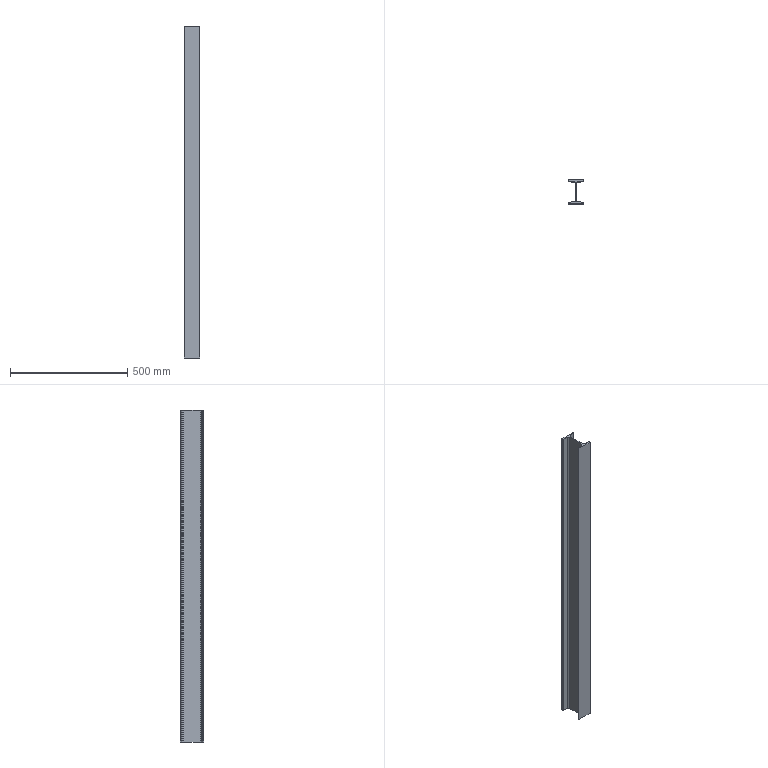Part | SolidWorks | features BaseBody 1 | 1 solid | 22 faces | box 67.6 x 101.6 x 1413 mm | volume 1963956 mm3 | plane 14 | cylinder 8 | commonest cylinder face diameters 5.6 x4 14.8 x4
STEP:
#1=CARTESIAN_POINT('',(45.812,22.014,0.));
#2=VERTEX_POINT('',#1);
#3=CARTESIAN_POINT('',(45.812,91.894,0.));
#4=VERTEX_POINT('',#3);
#5=CARTESIAN_POINT('',(45.812,91.894,0.));
#6=DIRECTION('',(0.,1.,0.));
#7=VECTOR('',#6,1000.);
#8=LINE('',#5,#7);
#9=EDGE_CURVE('',#2,#4,#8,.T.);
#10=ORIENTED_EDGE('',*,*,#9,.T.);
#11=CARTESIAN_POINT('',(45.812,91.894,1413.));
#12=VERTEX_POINT('',#11);
#13=CARTESIAN_POINT('',(45.812,91.894,0.));
#14=DIRECTION('',(0.,0.,1.));
#15=VECTOR('',#14,1000.);
#16=LINE('',#13,#15);
#17=EDGE_CURVE('',#4,#12,#16,.T.);
#18=ORIENTED_EDGE('',*,*,#17,.T.);
#19=CARTESIAN_POINT('',(45.812,22.014,1413.));
#20=VERTEX_POINT('',#19);
#21=CARTESIAN_POINT('',(45.812,91.894,1413.));
#22=DIRECTION('',(0.,-1.,0.));
#23=VECTOR('',#22,1000.);
#24=LINE('',#21,#23);
#25=EDGE_CURVE('',#12,#20,#24,.T.);
#26=ORIENTED_EDGE('',*,*,#25,.T.);
#27=CARTESIAN_POINT('',(45.812,22.014,0.));
#28=DIRECTION('',(0.,0.,-1.));
#29=VECTOR('',#28,1000.);
#30=LINE('',#27,#29);
#31=EDGE_CURVE('',#20,#2,#30,.T.);
#32=ORIENTED_EDGE('',*,*,#31,.T.);
#33=EDGE_LOOP('',(#10,#18,#26,#32));
#34=FACE_OUTER_BOUND('',#33,.T.);
#35=CARTESIAN_POINT('',(45.812,91.894,0.));
#36=DIRECTION('',(1.,0.,0.));
#37=DIRECTION('',(0.,0.,-1.));
#38=AXIS2_PLACEMENT_3D('',#35,#36,#37);
#39=PLANE('',#38);
#40=ADVANCED_FACE('',(#34),#39,.T.);
#41=ORIENTED_EDGE('',*,*,#17,.F.);
#42=CARTESIAN_POINT('',(51.991,99.193,0.));
#43=VERTEX_POINT('',#42);
#44=CARTESIAN_POINT('',(53.212,91.894,0.));
#45=DIRECTION('',(0.,0.,1.));
#46=DIRECTION('',(1.,0.,0.));
#47=AXIS2_PLACEMENT_3D('',#44,#45,#46);
#48=CIRCLE('',#47,7.4);
#49=EDGE_CURVE('',#43,#4,#48,.T.);
#50=ORIENTED_EDGE('',*,*,#49,.F.);
#51=CARTESIAN_POINT('',(51.991,99.193,1413.));
#52=VERTEX_POINT('',#51);
#53=CARTESIAN_POINT('',(51.991,99.193,0.));
#54=DIRECTION('',(0.,0.,-1.));
#55=VECTOR('',#54,1000.);
#56=LINE('',#53,#55);
#57=EDGE_CURVE('',#52,#43,#56,.T.);
#58=ORIENTED_EDGE('',*,*,#57,.F.);
#59=CARTESIAN_POINT('',(53.212,91.894,1413.));
#60=DIRECTION('',(0.,0.,-1.));
#61=DIRECTION('',(1.,0.,0.));
#62=AXIS2_PLACEMENT_3D('',#59,#60,#61);
#63=CIRCLE('',#62,7.4);
#64=EDGE_CURVE('',#12,#52,#63,.T.);
#65=ORIENTED_EDGE('',*,*,#64,.F.);
#66=EDGE_LOOP('',(#41,#50,#58,#65));
#67=FACE_OUTER_BOUND('',#66,.T.);
#68=CARTESIAN_POINT('',(53.212,91.894,0.));
#69=DIRECTION('',(0.,0.,1.));
#70=DIRECTION('',(1.,0.,0.));
#71=AXIS2_PLACEMENT_3D('',#68,#69,#70);
#72=CYLINDRICAL_SURFACE('',#71,7.4);
#73=ADVANCED_FACE('',(#67),#72,.F.);
#74=CARTESIAN_POINT('',(77.212,107.754,0.));
#75=VERTEX_POINT('',#74);
#76=CARTESIAN_POINT('',(9.612,107.754,0.));
#77=VERTEX_POINT('',#76);
#78=CARTESIAN_POINT('',(43.412,107.754,0.));
#79=DIRECTION('',(-1.,0.,0.));
#80=VECTOR('',#79,1000.);
#81=LINE('',#78,#80);
#82=EDGE_CURVE('',#75,#77,#81,.T.);
#83=ORIENTED_EDGE('',*,*,#82,.F.);
#84=CARTESIAN_POINT('',(77.212,105.784,0.));
#85=VERTEX_POINT('',#84);
#86=CARTESIAN_POINT('',(77.212,56.954,0.));
#87=DIRECTION('',(0.,1.,0.));
#88=VECTOR('',#87,1000.);
#89=LINE('',#86,#88);
#90=EDGE_CURVE('',#85,#75,#89,.T.);
#91=ORIENTED_EDGE('',*,*,#90,.F.);
#92=CARTESIAN_POINT('',(74.874,103.022,0.));
#93=VERTEX_POINT('',#92);
#94=CARTESIAN_POINT('',(74.412,105.784,0.));
#95=DIRECTION('',(0.,0.,1.));
#96=DIRECTION('',(1.,0.,0.));
#97=AXIS2_PLACEMENT_3D('',#94,#95,#96);
#98=CIRCLE('',#97,2.8);
#99=EDGE_CURVE('',#93,#85,#98,.T.);
#100=ORIENTED_EDGE('',*,*,#99,.F.);
#101=CARTESIAN_POINT('',(51.991,99.193,0.));
#102=DIRECTION('',(0.9863,0.165,0.));
#103=VECTOR('',#102,1000.);
#104=LINE('',#101,#103);
#105=EDGE_CURVE('',#43,#93,#104,.T.);
#106=ORIENTED_EDGE('',*,*,#105,.F.);
#107=ORIENTED_EDGE('',*,*,#49,.T.);
#108=ORIENTED_EDGE('',*,*,#9,.F.);
#109=CARTESIAN_POINT('',(51.991,14.716,0.));
#110=VERTEX_POINT('',#109);
#111=CARTESIAN_POINT('',(53.212,22.014,0.));
#112=DIRECTION('',(0.,0.,-1.));
#113=DIRECTION('',(1.,0.,0.));
#114=AXIS2_PLACEMENT_3D('',#111,#112,#113);
#115=CIRCLE('',#114,7.4);
#116=EDGE_CURVE('',#110,#2,#115,.T.);
#117=ORIENTED_EDGE('',*,*,#116,.F.);
#118=CARTESIAN_POINT('',(74.874,10.886,0.));
#119=VERTEX_POINT('',#118);
#120=CARTESIAN_POINT('',(74.874,10.886,0.));
#121=DIRECTION('',(-0.9863,0.165,0.));
#122=VECTOR('',#121,1000.);
#123=LINE('',#120,#122);
#124=EDGE_CURVE('',#119,#110,#123,.T.);
#125=ORIENTED_EDGE('',*,*,#124,.F.);
#126=CARTESIAN_POINT('',(77.212,8.125,0.));
#127=VERTEX_POINT('',#126);
#128=CARTESIAN_POINT('',(74.412,8.125,0.));
#129=DIRECTION('',(0.,0.,1.));
#130=DIRECTION('',(1.,0.,0.));
#131=AXIS2_PLACEMENT_3D('',#128,#129,#130);
#132=CIRCLE('',#131,2.8);
#133=EDGE_CURVE('',#127,#119,#132,.T.);
#134=ORIENTED_EDGE('',*,*,#133,.F.);
#135=CARTESIAN_POINT('',(77.212,6.154,0.));
#136=VERTEX_POINT('',#135);
#137=CARTESIAN_POINT('',(77.212,56.954,0.));
#138=DIRECTION('',(0.,1.,0.));
#139=VECTOR('',#138,1000.);
#140=LINE('',#137,#139);
#141=EDGE_CURVE('',#136,#127,#140,.T.);
#142=ORIENTED_EDGE('',*,*,#141,.F.);
#143=CARTESIAN_POINT('',(9.612,6.154,0.));
#144=VERTEX_POINT('',#143);
#145=CARTESIAN_POINT('',(43.412,6.154,0.));
#146=DIRECTION('',(1.,0.,0.));
#147=VECTOR('',#146,1000.);
#148=LINE('',#145,#147);
#149=EDGE_CURVE('',#144,#136,#148,.T.);
#150=ORIENTED_EDGE('',*,*,#149,.F.);
#151=CARTESIAN_POINT('',(9.612,8.125,0.));
#152=VERTEX_POINT('',#151);
#153=CARTESIAN_POINT('',(9.612,56.954,0.));
#154=DIRECTION('',(0.,-1.,0.));
#155=VECTOR('',#154,1000.);
#156=LINE('',#153,#155);
#157=EDGE_CURVE('',#152,#144,#156,.T.);
#158=ORIENTED_EDGE('',*,*,#157,.F.);
#159=CARTESIAN_POINT('',(11.95,10.886,0.));
#160=VERTEX_POINT('',#159);
#161=CARTESIAN_POINT('',(12.412,8.125,0.));
#162=DIRECTION('',(0.,0.,1.));
#163=DIRECTION('',(1.,0.,0.));
#164=AXIS2_PLACEMENT_3D('',#161,#162,#163);
#165=CIRCLE('',#164,2.8);
#166=EDGE_CURVE('',#160,#152,#165,.T.);
#167=ORIENTED_EDGE('',*,*,#166,.F.);
#168=CARTESIAN_POINT('',(34.833,14.716,0.));
#169=VERTEX_POINT('',#168);
#170=CARTESIAN_POINT('',(34.833,14.716,0.));
#171=DIRECTION('',(-0.9863,-0.165,0.));
#172=VECTOR('',#171,1000.);
#173=LINE('',#170,#172);
#174=EDGE_CURVE('',#169,#160,#173,.T.);
#175=ORIENTED_EDGE('',*,*,#174,.F.);
#176=CARTESIAN_POINT('',(41.012,22.014,0.));
#177=VERTEX_POINT('',#176);
#178=CARTESIAN_POINT('',(33.612,22.014,0.));
#179=DIRECTION('',(0.,0.,-1.));
#180=DIRECTION('',(1.,0.,0.));
#181=AXIS2_PLACEMENT_3D('',#178,#179,#180);
#182=CIRCLE('',#181,7.4);
#183=EDGE_CURVE('',#177,#169,#182,.T.);
#184=ORIENTED_EDGE('',*,*,#183,.F.);
#185=CARTESIAN_POINT('',(41.012,91.894,0.));
#186=VERTEX_POINT('',#185);
#187=CARTESIAN_POINT('',(41.012,56.954,0.));
#188=DIRECTION('',(0.,-1.,0.));
#189=VECTOR('',#188,1000.);
#190=LINE('',#187,#189);
#191=EDGE_CURVE('',#186,#177,#190,.T.);
#192=ORIENTED_EDGE('',*,*,#191,.F.);
#193=CARTESIAN_POINT('',(34.833,99.193,0.));
#194=VERTEX_POINT('',#193);
#195=CARTESIAN_POINT('',(33.612,91.894,0.));
#196=DIRECTION('',(0.,0.,-1.));
#197=DIRECTION('',(1.,0.,0.));
#198=AXIS2_PLACEMENT_3D('',#195,#196,#197);
#199=CIRCLE('',#198,7.4);
#200=EDGE_CURVE('',#194,#186,#199,.T.);
#201=ORIENTED_EDGE('',*,*,#200,.F.);
#202=CARTESIAN_POINT('',(11.95,103.022,0.));
#203=VERTEX_POINT('',#202);
#204=CARTESIAN_POINT('',(11.95,103.022,0.));
#205=DIRECTION('',(0.9863,-0.165,0.));
#206=VECTOR('',#205,1000.);
#207=LINE('',#204,#206);
#208=EDGE_CURVE('',#203,#194,#207,.T.);
#209=ORIENTED_EDGE('',*,*,#208,.F.);
#210=CARTESIAN_POINT('',(9.612,105.784,0.));
#211=VERTEX_POINT('',#210);
#212=CARTESIAN_POINT('',(12.412,105.784,0.));
#213=DIRECTION('',(0.,0.,1.));
#214=DIRECTION('',(1.,0.,0.));
#215=AXIS2_PLACEMENT_3D('',#212,#213,#214);
#216=CIRCLE('',#215,2.8);
#217=EDGE_CURVE('',#211,#203,#216,.T.);
#218=ORIENTED_EDGE('',*,*,#217,.F.);
#219=CARTESIAN_POINT('',(9.612,56.954,0.));
#220=DIRECTION('',(0.,-1.,0.));
#221=VECTOR('',#220,1000.);
#222=LINE('',#219,#221);
#223=EDGE_CURVE('',#77,#211,#222,.T.);
#224=ORIENTED_EDGE('',*,*,#223,.F.);
#225=EDGE_LOOP('',(#83,#91,#100,#106,#107,#108,#117,#125,#134,#142,#150,#158,#167,#175,#184,#192,#201,#209,#218,#224));
#226=FACE_OUTER_BOUND('',#225,.T.);
#227=CARTESIAN_POINT('',(43.412,56.954,0.));
#228=DIRECTION('',(0.,0.,1.));
#229=DIRECTION('',(1.,0.,0.));
#230=AXIS2_PLACEMENT_3D('',#227,#228,#229);
#231=PLANE('',#230);
#232=ADVANCED_FACE('',(#226),#231,.F.);
#233=CARTESIAN_POINT('',(51.991,14.716,1413.));
#234=VERTEX_POINT('',#233);
#235=CARTESIAN_POINT('',(51.991,14.716,0.));
#236=DIRECTION('',(0.,0.,1.));
#237=VECTOR('',#236,1000.);
#238=LINE('',#235,#237);
#239=EDGE_CURVE('',#110,#234,#238,.T.);
#240=ORIENTED_EDGE('',*,*,#239,.F.);
#241=ORIENTED_EDGE('',*,*,#116,.T.);
#242=ORIENTED_EDGE('',*,*,#31,.F.);
#243=CARTESIAN_POINT('',(53.212,22.014,1413.));
#244=DIRECTION('',(0.,0.,-1.));
#245=DIRECTION('',(1.,0.,0.));
#246=AXIS2_PLACEMENT_3D('',#243,#244,#245);
#247=CIRCLE('',#246,7.4);
#248=EDGE_CURVE('',#234,#20,#247,.T.);
#249=ORIENTED_EDGE('',*,*,#248,.F.);
#250=EDGE_LOOP('',(#240,#241,#242,#249));
#251=FACE_OUTER_BOUND('',#250,.T.);
#252=CARTESIAN_POINT('',(53.212,22.014,0.));
#253=DIRECTION('',(0.,0.,1.));
#254=DIRECTION('',(1.,0.,0.));
#255=AXIS2_PLACEMENT_3D('',#252,#253,#254);
#256=CYLINDRICAL_SURFACE('',#255,7.4);
#257=ADVANCED_FACE('',(#251),#256,.F.);
#258=CARTESIAN_POINT('',(74.874,103.022,1413.));
#259=VERTEX_POINT('',#258);
#260=CARTESIAN_POINT('',(77.212,105.784,1413.));
#261=VERTEX_POINT('',#260);
#262=CARTESIAN_POINT('',(74.412,105.784,1413.));
#263=DIRECTION('',(0.,0.,1.));
#264=DIRECTION('',(1.,0.,0.));
#265=AXIS2_PLACEMENT_3D('',#262,#263,#264);
#266=CIRCLE('',#265,2.8);
#267=EDGE_CURVE('',#259,#261,#266,.T.);
#268=ORIENTED_EDGE('',*,*,#267,.T.);
#269=CARTESIAN_POINT('',(77.212,107.754,1413.));
#270=VERTEX_POINT('',#269);
#271=CARTESIAN_POINT('',(77.212,56.954,1413.));
#272=DIRECTION('',(0.,1.,0.));
#273=VECTOR('',#272,1000.);
#274=LINE('',#271,#273);
#275=EDGE_CURVE('',#261,#270,#274,.T.);
#276=ORIENTED_EDGE('',*,*,#275,.T.);
#277=CARTESIAN_POINT('',(9.612,107.754,1413.));
#278=VERTEX_POINT('',#277);
#279=CARTESIAN_POINT('',(43.412,107.754,1413.));
#280=DIRECTION('',(-1.,0.,0.));
#281=VECTOR('',#280,1000.);
#282=LINE('',#279,#281);
#283=EDGE_CURVE('',#270,#278,#282,.T.);
#284=ORIENTED_EDGE('',*,*,#283,.T.);
#285=CARTESIAN_POINT('',(9.612,105.784,1413.));
#286=VERTEX_POINT('',#285);
#287=CARTESIAN_POINT('',(9.612,56.954,1413.));
#288=DIRECTION('',(0.,-1.,0.));
#289=VECTOR('',#288,1000.);
#290=LINE('',#287,#289);
#291=EDGE_CURVE('',#278,#286,#290,.T.);
#292=ORIENTED_EDGE('',*,*,#291,.T.);
#293=CARTESIAN_POINT('',(11.95,103.022,1413.));
#294=VERTEX_POINT('',#293);
#295=CARTESIAN_POINT('',(12.412,105.784,1413.));
#296=DIRECTION('',(0.,0.,1.));
#297=DIRECTION('',(1.,0.,0.));
#298=AXIS2_PLACEMENT_3D('',#295,#296,#297);
#299=CIRCLE('',#298,2.8);
#300=EDGE_CURVE('',#286,#294,#299,.T.);
#301=ORIENTED_EDGE('',*,*,#300,.T.);
#302=CARTESIAN_POINT('',(34.833,99.193,1413.));
#303=VERTEX_POINT('',#302);
#304=CARTESIAN_POINT('',(11.95,103.022,1413.));
#305=DIRECTION('',(0.9863,-0.165,0.));
#306=VECTOR('',#305,1000.);
#307=LINE('',#304,#306);
#308=EDGE_CURVE('',#294,#303,#307,.T.);
#309=ORIENTED_EDGE('',*,*,#308,.T.);
#310=CARTESIAN_POINT('',(41.012,91.894,1413.));
#311=VERTEX_POINT('',#310);
#312=CARTESIAN_POINT('',(33.612,91.894,1413.));
#313=DIRECTION('',(0.,0.,-1.));
#314=DIRECTION('',(1.,0.,0.));
#315=AXIS2_PLACEMENT_3D('',#312,#313,#314);
#316=CIRCLE('',#315,7.4);
#317=EDGE_CURVE('',#303,#311,#316,.T.);
#318=ORIENTED_EDGE('',*,*,#317,.T.);
#319=CARTESIAN_POINT('',(41.012,22.014,1413.));
#320=VERTEX_POINT('',#319);
#321=CARTESIAN_POINT('',(41.012,56.954,1413.));
#322=DIRECTION('',(0.,-1.,0.));
#323=VECTOR('',#322,1000.);
#324=LINE('',#321,#323);
#325=EDGE_CURVE('',#311,#320,#324,.T.);
#326=ORIENTED_EDGE('',*,*,#325,.T.);
#327=CARTESIAN_POINT('',(34.833,14.716,1413.));
#328=VERTEX_POINT('',#327);
#329=CARTESIAN_POINT('',(33.612,22.014,1413.));
#330=DIRECTION('',(0.,0.,-1.));
#331=DIRECTION('',(1.,0.,0.));
#332=AXIS2_PLACEMENT_3D('',#329,#330,#331);
#333=CIRCLE('',#332,7.4);
#334=EDGE_CURVE('',#320,#328,#333,.T.);
#335=ORIENTED_EDGE('',*,*,#334,.T.);
#336=CARTESIAN_POINT('',(11.95,10.886,1413.));
#337=VERTEX_POINT('',#336);
#338=CARTESIAN_POINT('',(34.833,14.716,1413.));
#339=DIRECTION('',(-0.9863,-0.165,0.));
#340=VECTOR('',#339,1000.);
#341=LINE('',#338,#340);
#342=EDGE_CURVE('',#328,#337,#341,.T.);
#343=ORIENTED_EDGE('',*,*,#342,.T.);
#344=CARTESIAN_POINT('',(9.612,8.125,1413.));
#345=VERTEX_POINT('',#344);
#346=CARTESIAN_POINT('',(12.412,8.125,1413.));
#347=DIRECTION('',(0.,0.,1.));
#348=DIRECTION('',(1.,0.,0.));
#349=AXIS2_PLACEMENT_3D('',#346,#347,#348);
#350=CIRCLE('',#349,2.8);
#351=EDGE_CURVE('',#337,#345,#350,.T.);
#352=ORIENTED_EDGE('',*,*,#351,.T.);
#353=CARTESIAN_POINT('',(9.612,6.154,1413.));
#354=VERTEX_POINT('',#353);
#355=CARTESIAN_POINT('',(9.612,56.954,1413.));
#356=DIRECTION('',(0.,-1.,0.));
#357=VECTOR('',#356,1000.);
#358=LINE('',#355,#357);
#359=EDGE_CURVE('',#345,#354,#358,.T.);
#360=ORIENTED_EDGE('',*,*,#359,.T.);
#361=CARTESIAN_POINT('',(77.212,6.154,1413.));
#362=VERTEX_POINT('',#361);
#363=CARTESIAN_POINT('',(43.412,6.154,1413.));
#364=DIRECTION('',(1.,0.,0.));
#365=VECTOR('',#364,1000.);
#366=LINE('',#363,#365);
#367=EDGE_CURVE('',#354,#362,#366,.T.);
#368=ORIENTED_EDGE('',*,*,#367,.T.);
#369=CARTESIAN_POINT('',(77.212,8.125,1413.));
#370=VERTEX_POINT('',#369);
#371=CARTESIAN_POINT('',(77.212,56.954,1413.));
#372=DIRECTION('',(0.,1.,0.));
#373=VECTOR('',#372,1000.);
#374=LINE('',#371,#373);
#375=EDGE_CURVE('',#362,#370,#374,.T.);
#376=ORIENTED_EDGE('',*,*,#375,.T.);
#377=CARTESIAN_POINT('',(74.874,10.886,1413.));
#378=VERTEX_POINT('',#377);
#379=CARTESIAN_POINT('',(74.412,8.125,1413.));
#380=DIRECTION('',(0.,0.,1.));
#381=DIRECTION('',(1.,0.,0.));
#382=AXIS2_PLACEMENT_3D('',#379,#380,#381);
#383=CIRCLE('',#382,2.8);
#384=EDGE_CURVE('',#370,#378,#383,.T.);
#385=ORIENTED_EDGE('',*,*,#384,.T.);
#386=CARTESIAN_POINT('',(74.874,10.886,1413.));
#387=DIRECTION('',(-0.9863,0.165,0.));
#388=VECTOR('',#387,1000.);
#389=LINE('',#386,#388);
#390=EDGE_CURVE('',#378,#234,#389,.T.);
#391=ORIENTED_EDGE('',*,*,#390,.T.);
#392=ORIENTED_EDGE('',*,*,#248,.T.);
#393=ORIENTED_EDGE('',*,*,#25,.F.);
#394=ORIENTED_EDGE('',*,*,#64,.T.);
#395=CARTESIAN_POINT('',(51.991,99.193,1413.));
#396=DIRECTION('',(0.9863,0.165,0.));
#397=VECTOR('',#396,1000.);
#398=LINE('',#395,#397);
#399=EDGE_CURVE('',#52,#259,#398,.T.);
#400=ORIENTED_EDGE('',*,*,#399,.T.);
#401=EDGE_LOOP('',(#268,#276,#284,#292,#301,#309,#318,#326,#335,#343,#352,#360,#368,#376,#385,#391,#392,#393,#394,#400));
#402=FACE_OUTER_BOUND('',#401,.T.);
#403=CARTESIAN_POINT('',(43.412,56.954,1413.));
#404=DIRECTION('',(0.,0.,1.));
#405=DIRECTION('',(1.,0.,0.));
#406=AXIS2_PLACEMENT_3D('',#403,#404,#405);
#407=PLANE('',#406);
#408=ADVANCED_FACE('',(#402),#407,.T.);
#409=ORIENTED_EDGE('',*,*,#105,.T.);
#410=CARTESIAN_POINT('',(74.874,103.022,0.));
#411=DIRECTION('',(0.,0.,1.));
#412=VECTOR('',#411,1000.);
#413=LINE('',#410,#412);
#414=EDGE_CURVE('',#93,#259,#413,.T.);
#415=ORIENTED_EDGE('',*,*,#414,.T.);
#416=ORIENTED_EDGE('',*,*,#399,.F.);
#417=ORIENTED_EDGE('',*,*,#57,.T.);
#418=EDGE_LOOP('',(#409,#415,#416,#417));
#419=FACE_OUTER_BOUND('',#418,.T.);
#420=CARTESIAN_POINT('',(74.874,103.022,0.));
#421=DIRECTION('',(0.165,-0.9863,0.));
#422=DIRECTION('',(0.9863,0.165,0.));
#423=AXIS2_PLACEMENT_3D('',#420,#421,#422);
#424=PLANE('',#423);
#425=ADVANCED_FACE('',(#419),#424,.T.);
#426=ORIENTED_EDGE('',*,*,#223,.T.);
#427=CARTESIAN_POINT('',(9.612,105.784,0.));
#428=DIRECTION('',(0.,0.,1.));
#429=VECTOR('',#428,1000.);
#430=LINE('',#427,#429);
#431=EDGE_CURVE('',#211,#286,#430,.T.);
#432=ORIENTED_EDGE('',*,*,#431,.T.);
#433=ORIENTED_EDGE('',*,*,#291,.F.);
#434=CARTESIAN_POINT('',(9.612,107.754,0.));
#435=DIRECTION('',(0.,0.,-1.));
#436=VECTOR('',#435,1000.);
#437=LINE('',#434,#436);
#438=EDGE_CURVE('',#278,#77,#437,.T.);
#439=ORIENTED_EDGE('',*,*,#438,.T.);
#440=EDGE_LOOP('',(#426,#432,#433,#439));
#441=FACE_OUTER_BOUND('',#440,.T.);
#442=CARTESIAN_POINT('',(9.612,105.784,0.));
#443=DIRECTION('',(-1.,0.,0.));
#444=DIRECTION('',(0.,0.,1.));
#445=AXIS2_PLACEMENT_3D('',#442,#443,#444);
#446=PLANE('',#445);
#447=ADVANCED_FACE('',(#441),#446,.T.);
#448=ORIENTED_EDGE('',*,*,#82,.T.);
#449=ORIENTED_EDGE('',*,*,#438,.F.);
#450=ORIENTED_EDGE('',*,*,#283,.F.);
#451=CARTESIAN_POINT('',(77.212,107.754,0.));
#452=DIRECTION('',(0.,0.,-1.));
#453=VECTOR('',#452,1000.);
#454=LINE('',#451,#453);
#455=EDGE_CURVE('',#270,#75,#454,.T.);
#456=ORIENTED_EDGE('',*,*,#455,.T.);
#457=EDGE_LOOP('',(#448,#449,#450,#456));
#458=FACE_OUTER_BOUND('',#457,.T.);
#459=CARTESIAN_POINT('',(9.612,107.754,0.));
#460=DIRECTION('',(0.,1.,0.));
#461=DIRECTION('',(0.,0.,1.));
#462=AXIS2_PLACEMENT_3D('',#459,#460,#461);
#463=PLANE('',#462);
#464=ADVANCED_FACE('',(#458),#463,.T.);
#465=ORIENTED_EDGE('',*,*,#90,.T.);
#466=ORIENTED_EDGE('',*,*,#455,.F.);
#467=ORIENTED_EDGE('',*,*,#275,.F.);
#468=CARTESIAN_POINT('',(77.212,105.784,0.));
#469=DIRECTION('',(0.,0.,-1.));
#470=VECTOR('',#469,1000.);
#471=LINE('',#468,#470);
#472=EDGE_CURVE('',#261,#85,#471,.T.);
#473=ORIENTED_EDGE('',*,*,#472,.T.);
#474=EDGE_LOOP('',(#465,#466,#467,#473));
#475=FACE_OUTER_BOUND('',#474,.T.);
#476=CARTESIAN_POINT('',(77.212,107.754,0.));
#477=DIRECTION('',(1.,0.,0.));
#478=DIRECTION('',(0.,1.,0.));
#479=AXIS2_PLACEMENT_3D('',#476,#477,#478);
#480=PLANE('',#479);
#481=ADVANCED_FACE('',(#475),#480,.T.);
#482=ORIENTED_EDGE('',*,*,#99,.T.);
#483=ORIENTED_EDGE('',*,*,#472,.F.);
#484=ORIENTED_EDGE('',*,*,#267,.F.);
#485=ORIENTED_EDGE('',*,*,#414,.F.);
#486=EDGE_LOOP('',(#482,#483,#484,#485));
#487=FACE_OUTER_BOUND('',#486,.T.);
#488=CARTESIAN_POINT('',(74.412,105.784,0.));
#489=DIRECTION('',(0.,0.,1.));
#490=DIRECTION('',(1.,0.,0.));
#491=AXIS2_PLACEMENT_3D('',#488,#489,#490);
#492=CYLINDRICAL_SURFACE('',#491,2.8);
#493=ADVANCED_FACE('',(#487),#492,.T.);
#494=ORIENTED_EDGE('',*,*,#124,.T.);
#495=ORIENTED_EDGE('',*,*,#239,.T.);
#496=ORIENTED_EDGE('',*,*,#390,.F.);
#497=CARTESIAN_POINT('',(74.874,10.886,0.));
#498=DIRECTION('',(0.,0.,-1.));
#499=VECTOR('',#498,1000.);
#500=LINE('',#497,#499);
#501=EDGE_CURVE('',#378,#119,#500,.T.);
#502=ORIENTED_EDGE('',*,*,#501,.T.);
#503=EDGE_LOOP('',(#494,#495,#496,#502));
#504=FACE_OUTER_BOUND('',#503,.T.);
#505=CARTESIAN_POINT('',(51.991,14.716,0.));
#506=DIRECTION('',(0.165,0.9863,0.));
#507=DIRECTION('',(-0.9863,0.165,0.));
#508=AXIS2_PLACEMENT_3D('',#505,#506,#507);
#509=PLANE('',#508);
#510=ADVANCED_FACE('',(#504),#509,.T.);
#511=ORIENTED_EDGE('',*,*,#133,.T.);
#512=ORIENTED_EDGE('',*,*,#501,.F.);
#513=ORIENTED_EDGE('',*,*,#384,.F.);
#514=CARTESIAN_POINT('',(77.212,8.125,0.));
#515=DIRECTION('',(0.,0.,-1.));
#516=VECTOR('',#515,1000.);
#517=LINE('',#514,#516);
#518=EDGE_CURVE('',#370,#127,#517,.T.);
#519=ORIENTED_EDGE('',*,*,#518,.T.);
#520=EDGE_LOOP('',(#511,#512,#513,#519));
#521=FACE_OUTER_BOUND('',#520,.T.);
#522=CARTESIAN_POINT('',(74.412,8.125,0.));
#523=DIRECTION('',(0.,0.,1.));
#524=DIRECTION('',(1.,0.,0.));
#525=AXIS2_PLACEMENT_3D('',#522,#523,#524);
#526=CYLINDRICAL_SURFACE('',#525,2.8);
#527=ADVANCED_FACE('',(#521),#526,.T.);
#528=ORIENTED_EDGE('',*,*,#141,.T.);
#529=ORIENTED_EDGE('',*,*,#518,.F.);
#530=ORIENTED_EDGE('',*,*,#375,.F.);
#531=CARTESIAN_POINT('',(77.212,6.154,0.));
#532=DIRECTION('',(0.,0.,-1.));
#533=VECTOR('',#532,1000.);
#534=LINE('',#531,#533);
#535=EDGE_CURVE('',#362,#136,#534,.T.);
#536=ORIENTED_EDGE('',*,*,#535,.T.);
#537=EDGE_LOOP('',(#528,#529,#530,#536));
#538=FACE_OUTER_BOUND('',#537,.T.);
#539=CARTESIAN_POINT('',(77.212,8.125,0.));
#540=DIRECTION('',(1.,0.,0.));
#541=DIRECTION('',(0.,1.,0.));
#542=AXIS2_PLACEMENT_3D('',#539,#540,#541);
#543=PLANE('',#542);
#544=ADVANCED_FACE('',(#538),#543,.T.);
#545=ORIENTED_EDGE('',*,*,#149,.T.);
#546=ORIENTED_EDGE('',*,*,#535,.F.);
#547=ORIENTED_EDGE('',*,*,#367,.F.);
#548=CARTESIAN_POINT('',(9.612,6.154,0.));
#549=DIRECTION('',(0.,0.,-1.));
#550=VECTOR('',#549,1000.);
#551=LINE('',#548,#550);
#552=EDGE_CURVE('',#354,#144,#551,.T.);
#553=ORIENTED_EDGE('',*,*,#552,.T.);
#554=EDGE_LOOP('',(#545,#546,#547,#553));
#555=FACE_OUTER_BOUND('',#554,.T.);
#556=CARTESIAN_POINT('',(77.212,6.154,0.));
#557=DIRECTION('',(0.,-1.,0.));
#558=DIRECTION('',(0.,0.,-1.));
#559=AXIS2_PLACEMENT_3D('',#556,#557,#558);
#560=PLANE('',#559);
#561=ADVANCED_FACE('',(#555),#560,.T.);
#562=ORIENTED_EDGE('',*,*,#157,.T.);
#563=ORIENTED_EDGE('',*,*,#552,.F.);
#564=ORIENTED_EDGE('',*,*,#359,.F.);
#565=CARTESIAN_POINT('',(9.612,8.125,0.));
#566=DIRECTION('',(0.,0.,-1.));
#567=VECTOR('',#566,1000.);
#568=LINE('',#565,#567);
#569=EDGE_CURVE('',#345,#152,#568,.T.);
#570=ORIENTED_EDGE('',*,*,#569,.T.);
#571=EDGE_LOOP('',(#562,#563,#564,#570));
#572=FACE_OUTER_BOUND('',#571,.T.);
#573=CARTESIAN_POINT('',(9.612,6.154,0.));
#574=DIRECTION('',(-1.,0.,0.));
#575=DIRECTION('',(0.,-1.,0.));
#576=AXIS2_PLACEMENT_3D('',#573,#574,#575);
#577=PLANE('',#576);
#578=ADVANCED_FACE('',(#572),#577,.T.);
#579=ORIENTED_EDGE('',*,*,#166,.T.);
#580=ORIENTED_EDGE('',*,*,#569,.F.);
#581=ORIENTED_EDGE('',*,*,#351,.F.);
#582=CARTESIAN_POINT('',(11.95,10.886,0.));
#583=DIRECTION('',(0.,0.,-1.));
#584=VECTOR('',#583,1000.);
#585=LINE('',#582,#584);
#586=EDGE_CURVE('',#337,#160,#585,.T.);
#587=ORIENTED_EDGE('',*,*,#586,.T.);
#588=EDGE_LOOP('',(#579,#580,#581,#587));
#589=FACE_OUTER_BOUND('',#588,.T.);
#590=CARTESIAN_POINT('',(12.412,8.125,0.));
#591=DIRECTION('',(0.,0.,1.));
#592=DIRECTION('',(1.,0.,0.));
#593=AXIS2_PLACEMENT_3D('',#590,#591,#592);
#594=CYLINDRICAL_SURFACE('',#593,2.8);
#595=ADVANCED_FACE('',(#589),#594,.T.);
#596=ORIENTED_EDGE('',*,*,#174,.T.);
#597=ORIENTED_EDGE('',*,*,#586,.F.);
#598=ORIENTED_EDGE('',*,*,#342,.F.);
#599=CARTESIAN_POINT('',(34.833,14.716,0.));
#600=DIRECTION('',(0.,0.,-1.));
#601=VECTOR('',#600,1000.);
#602=LINE('',#599,#601);
#603=EDGE_CURVE('',#328,#169,#602,.T.);
#604=ORIENTED_EDGE('',*,*,#603,.T.);
#605=EDGE_LOOP('',(#596,#597,#598,#604));
#606=FACE_OUTER_BOUND('',#605,.T.);
#607=CARTESIAN_POINT('',(11.95,10.886,0.));
#608=DIRECTION('',(-0.165,0.9863,0.));
#609=DIRECTION('',(-0.9863,-0.165,0.));
#610=AXIS2_PLACEMENT_3D('',#607,#608,#609);
#611=PLANE('',#610);
#612=ADVANCED_FACE('',(#606),#611,.T.);
#613=CARTESIAN_POINT('',(41.012,22.014,0.));
#614=DIRECTION('',(0.,0.,1.));
#615=VECTOR('',#614,1000.);
#616=LINE('',#613,#615);
#617=EDGE_CURVE('',#177,#320,#616,.T.);
#618=ORIENTED_EDGE('',*,*,#617,.F.);
#619=ORIENTED_EDGE('',*,*,#183,.T.);
#620=ORIENTED_EDGE('',*,*,#603,.F.);
#621=ORIENTED_EDGE('',*,*,#334,.F.);
#622=EDGE_LOOP('',(#618,#619,#620,#621));
#623=FACE_OUTER_BOUND('',#622,.T.);
#624=CARTESIAN_POINT('',(33.612,22.014,0.));
#625=DIRECTION('',(0.,0.,1.));
#626=DIRECTION('',(1.,0.,0.));
#627=AXIS2_PLACEMENT_3D('',#624,#625,#626);
#628=CYLINDRICAL_SURFACE('',#627,7.4);
#629=ADVANCED_FACE('',(#623),#628,.F.);
#630=ORIENTED_EDGE('',*,*,#191,.T.);
#631=ORIENTED_EDGE('',*,*,#617,.T.);
#632=ORIENTED_EDGE('',*,*,#325,.F.);
#633=CARTESIAN_POINT('',(41.012,91.894,0.));
#634=DIRECTION('',(0.,0.,-1.));
#635=VECTOR('',#634,1000.);
#636=LINE('',#633,#635);
#637=EDGE_CURVE('',#311,#186,#636,.T.);
#638=ORIENTED_EDGE('',*,*,#637,.T.);
#639=EDGE_LOOP('',(#630,#631,#632,#638));
#640=FACE_OUTER_BOUND('',#639,.T.);
#641=CARTESIAN_POINT('',(41.012,22.014,0.));
#642=DIRECTION('',(-1.,0.,0.));
#643=DIRECTION('',(0.,0.,1.));
#644=AXIS2_PLACEMENT_3D('',#641,#642,#643);
#645=PLANE('',#644);
#646=ADVANCED_FACE('',(#640),#645,.T.);
#647=CARTESIAN_POINT('',(34.833,99.193,0.));
#648=DIRECTION('',(0.,0.,1.));
#649=VECTOR('',#648,1000.);
#650=LINE('',#647,#649);
#651=EDGE_CURVE('',#194,#303,#650,.T.);
#652=ORIENTED_EDGE('',*,*,#651,.F.);
#653=ORIENTED_EDGE('',*,*,#200,.T.);
#654=ORIENTED_EDGE('',*,*,#637,.F.);
#655=ORIENTED_EDGE('',*,*,#317,.F.);
#656=EDGE_LOOP('',(#652,#653,#654,#655));
#657=FACE_OUTER_BOUND('',#656,.T.);
#658=CARTESIAN_POINT('',(33.612,91.894,0.));
#659=DIRECTION('',(0.,0.,1.));
#660=DIRECTION('',(1.,0.,0.));
#661=AXIS2_PLACEMENT_3D('',#658,#659,#660);
#662=CYLINDRICAL_SURFACE('',#661,7.4);
#663=ADVANCED_FACE('',(#657),#662,.F.);
#664=ORIENTED_EDGE('',*,*,#208,.T.);
#665=ORIENTED_EDGE('',*,*,#651,.T.);
#666=ORIENTED_EDGE('',*,*,#308,.F.);
#667=CARTESIAN_POINT('',(11.95,103.022,0.));
#668=DIRECTION('',(0.,0.,-1.));
#669=VECTOR('',#668,1000.);
#670=LINE('',#667,#669);
#671=EDGE_CURVE('',#294,#203,#670,.T.);
#672=ORIENTED_EDGE('',*,*,#671,.T.);
#673=EDGE_LOOP('',(#664,#665,#666,#672));
#674=FACE_OUTER_BOUND('',#673,.T.);
#675=CARTESIAN_POINT('',(34.833,99.193,0.));
#676=DIRECTION('',(-0.165,-0.9863,0.));
#677=DIRECTION('',(0.9863,-0.165,0.));
#678=AXIS2_PLACEMENT_3D('',#675,#676,#677);
#679=PLANE('',#678);
#680=ADVANCED_FACE('',(#674),#679,.T.);
#681=ORIENTED_EDGE('',*,*,#217,.T.);
#682=ORIENTED_EDGE('',*,*,#671,.F.);
#683=ORIENTED_EDGE('',*,*,#300,.F.);
#684=ORIENTED_EDGE('',*,*,#431,.F.);
#685=EDGE_LOOP('',(#681,#682,#683,#684));
#686=FACE_OUTER_BOUND('',#685,.T.);
#687=CARTESIAN_POINT('',(12.412,105.784,0.));
#688=DIRECTION('',(0.,0.,1.));
#689=DIRECTION('',(1.,0.,0.));
#690=AXIS2_PLACEMENT_3D('',#687,#688,#689);
#691=CYLINDRICAL_SURFACE('',#690,2.8);
#692=ADVANCED_FACE('',(#686),#691,.T.);
#693=CLOSED_SHELL('',(#40,#73,#232,#257,#408,#425,#447,#464,#481,#493,#510,#527,#544,#561,#578,#595,#612,#629,#646,#663,#680,#692));
#694=MANIFOLD_SOLID_BREP('',#693);
#695=CARTESIAN_POINT('',(0.,0.,0.));
#696=DIRECTION('',(0.,0.,1.));
#697=DIRECTION('',(1.,0.,0.));
#698=AXIS2_PLACEMENT_3D('',#695,#696,#697);
#699=(LENGTH_UNIT()NAMED_UNIT(*)SI_UNIT(.MILLI.,.METRE.));
#700=UNCERTAINTY_MEASURE_WITH_UNIT(LENGTH_MEASURE(0.00001),#699,'','');
#701=(NAMED_UNIT(*)PLANE_ANGLE_UNIT()SI_UNIT($,.RADIAN.));
#702=(NAMED_UNIT(*)SI_UNIT($,.STERADIAN.)SOLID_ANGLE_UNIT());
#703=(GEOMETRIC_REPRESENTATION_CONTEXT(3)GLOBAL_UNCERTAINTY_ASSIGNED_CONTEXT((#700))GLOBAL_UNIT_ASSIGNED_CONTEXT((#699,#701,#702))REPRESENTATION_CONTEXT('',''));
#704=ADVANCED_BREP_SHAPE_REPRESENTATION('',(#694,#698),#703);